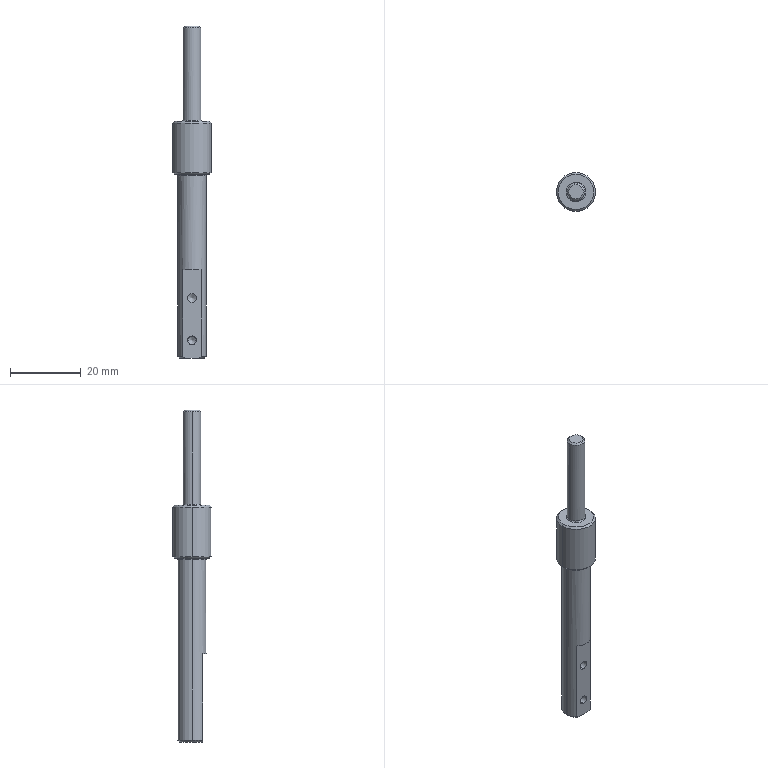Part | STEP file | Conductive post-PN_0001 | 1 solid | 33 faces | box 11 x 11 x 94 mm | volume 4420 mm3 | cone 13 | cylinder 10 | plane 6 | spline 4 | commonest cylinder face diameters 2.5 x4 5 x2 8 x2 11 x2